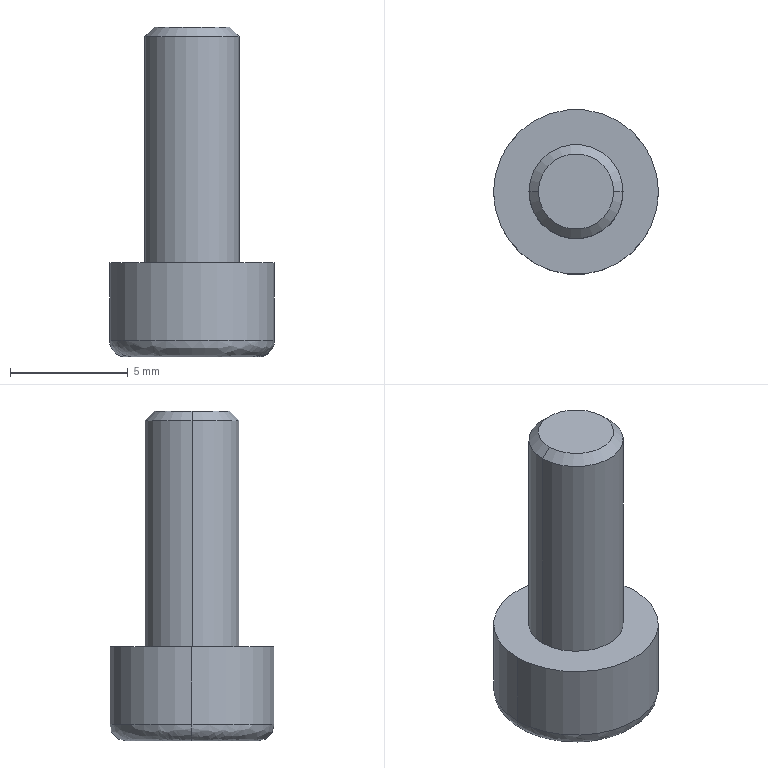Part | STEP file | LE-YZS-M4X10_PN_0007 | 1 solid | 25 faces | box 7 x 7 x 14 mm | volume 258.83 mm3 | plane 15 | cylinder 4 | cone 4 | spline 2 | commonest cylinder face diameters 4 x2 7 x2
STEP:
#1=CARTESIAN_POINT('',(-3.5,0.,-3.3));
#2=VERTEX_POINT('',#1);
#3=CARTESIAN_POINT('',(3.5,0.,-3.3));
#4=VERTEX_POINT('',#3);
#5=CARTESIAN_POINT('',(0.,0.,-3.3));
#6=DIRECTION('',(0.,0.,1.));
#7=DIRECTION('',(1.,0.,0.));
#8=AXIS2_PLACEMENT_3D('',#5,#6,#7);
#9=CIRCLE('',#8,3.5);
#10=EDGE_CURVE('',#2,#4,#9,.T.);
#11=ORIENTED_EDGE('',*,*,#10,.F.);
#12=CARTESIAN_POINT('',(-2.8,0.,-4.));
#13=VERTEX_POINT('',#12);
#14=CARTESIAN_POINT('',(-2.8,0.,-3.3));
#15=DIRECTION('',(0.,-1.,0.));
#16=DIRECTION('',(-1.,0.,0.));
#17=AXIS2_PLACEMENT_3D('',#14,#15,#16);
#18=CIRCLE('',#17,0.7);
#19=EDGE_CURVE('',#2,#13,#18,.T.);
#20=ORIENTED_EDGE('',*,*,#19,.T.);
#21=CARTESIAN_POINT('',(2.8,0.,-4.));
#22=VERTEX_POINT('',#21);
#23=CARTESIAN_POINT('',(-2.8,0.,-4.));
#24=CARTESIAN_POINT('',(-2.8,-5.6,-4.));
#25=CARTESIAN_POINT('',(2.8,-5.6,-4.));
#26=CARTESIAN_POINT('',(2.8,0.,-4.));
#27=(BOUNDED_CURVE()B_SPLINE_CURVE(3,(#23,#24,#25,#26),.UNSPECIFIED.,.F.,.F.)B_SPLINE_CURVE_WITH_KNOTS((4,4),(0.,1.),.UNSPECIFIED.)CURVE()GEOMETRIC_REPRESENTATION_ITEM()RATIONAL_B_SPLINE_CURVE((1.,0.3333,0.3333,1.))REPRESENTATION_ITEM(''));
#28=EDGE_CURVE('',#13,#22,#27,.T.);
#29=ORIENTED_EDGE('',*,*,#28,.T.);
#30=CARTESIAN_POINT('',(2.8,0.,-3.3));
#31=DIRECTION('',(0.,1.,0.));
#32=DIRECTION('',(1.,0.,0.));
#33=AXIS2_PLACEMENT_3D('',#30,#31,#32);
#34=CIRCLE('',#33,0.7);
#35=EDGE_CURVE('',#4,#22,#34,.T.);
#36=ORIENTED_EDGE('',*,*,#35,.F.);
#37=EDGE_LOOP('',(#11,#20,#29,#36));
#38=FACE_OUTER_BOUND('',#37,.T.);
#39=CARTESIAN_POINT('',(-3.5,0.,-3.3));
#40=CARTESIAN_POINT('',(-3.5,-7.,-3.3));
#41=CARTESIAN_POINT('',(3.5,-7.,-3.3));
#42=CARTESIAN_POINT('',(3.5,0.,-3.3));
#43=CARTESIAN_POINT('',(-3.5,0.,-3.71));
#44=CARTESIAN_POINT('',(-3.5,-7.,-3.71));
#45=CARTESIAN_POINT('',(3.5,-7.,-3.71));
#46=CARTESIAN_POINT('',(3.5,0.,-3.71));
#47=CARTESIAN_POINT('',(-3.21,0.,-4.));
#48=CARTESIAN_POINT('',(-3.21,-6.42,-4.));
#49=CARTESIAN_POINT('',(3.21,-6.42,-4.));
#50=CARTESIAN_POINT('',(3.21,0.,-4.));
#51=CARTESIAN_POINT('',(-2.8,0.,-4.));
#52=CARTESIAN_POINT('',(-2.8,-5.6,-4.));
#53=CARTESIAN_POINT('',(2.8,-5.6,-4.));
#54=CARTESIAN_POINT('',(2.8,0.,-4.));
#55=(BOUNDED_SURFACE()B_SPLINE_SURFACE(3,3,((#39,#40,#41,#42),(#43,#44,#45,#46),(#47,#48,#49,#50),(#51,#52,#53,#54)),.UNSPECIFIED.,.F.,.F.,.T.)B_SPLINE_SURFACE_WITH_KNOTS((4,4),(4,4),(0.,1.),(0.,1.),.UNSPECIFIED.)GEOMETRIC_REPRESENTATION_ITEM()RATIONAL_B_SPLINE_SURFACE(((1.,0.3333,0.3333,1.),(0.8047,0.2682,0.2682,0.8047),(0.8047,0.2682,0.2682,0.8047),(1.,0.3333,0.3333,1.)))REPRESENTATION_ITEM('')SURFACE());
#56=ADVANCED_FACE('',(#38),#55,.T.);
#57=CARTESIAN_POINT('',(-2.,0.,9.6));
#58=VERTEX_POINT('',#57);
#59=CARTESIAN_POINT('',(2.,0.,9.6));
#60=VERTEX_POINT('',#59);
#61=CARTESIAN_POINT('',(0.,0.,9.6));
#62=DIRECTION('',(0.,0.,-1.));
#63=DIRECTION('',(-1.,0.,0.));
#64=AXIS2_PLACEMENT_3D('',#61,#62,#63);
#65=CIRCLE('',#64,2.);
#66=EDGE_CURVE('',#58,#60,#65,.T.);
#67=ORIENTED_EDGE('',*,*,#66,.T.);
#68=CARTESIAN_POINT('',(2.,0.,0.));
#69=VERTEX_POINT('',#68);
#70=CARTESIAN_POINT('',(2.,0.,10.));
#71=DIRECTION('',(0.,0.,-1.));
#72=VECTOR('',#71,1000.);
#73=LINE('',#70,#72);
#74=EDGE_CURVE('',#60,#69,#73,.T.);
#75=ORIENTED_EDGE('',*,*,#74,.T.);
#76=CARTESIAN_POINT('',(-2.,0.,0.));
#77=VERTEX_POINT('',#76);
#78=CARTESIAN_POINT('',(0.,0.,0.));
#79=DIRECTION('',(0.,0.,1.));
#80=DIRECTION('',(-1.,0.,0.));
#81=AXIS2_PLACEMENT_3D('',#78,#79,#80);
#82=CIRCLE('',#81,2.);
#83=EDGE_CURVE('',#69,#77,#82,.T.);
#84=ORIENTED_EDGE('',*,*,#83,.T.);
#85=CARTESIAN_POINT('',(-2.,0.,10.));
#86=DIRECTION('',(0.,0.,-1.));
#87=VECTOR('',#86,1000.);
#88=LINE('',#85,#87);
#89=EDGE_CURVE('',#58,#77,#88,.T.);
#90=ORIENTED_EDGE('',*,*,#89,.F.);
#91=EDGE_LOOP('',(#67,#75,#84,#90));
#92=FACE_OUTER_BOUND('',#91,.T.);
#93=CARTESIAN_POINT('',(0.,0.,10.));
#94=DIRECTION('',(0.,0.,-1.));
#95=DIRECTION('',(-1.,0.,0.));
#96=AXIS2_PLACEMENT_3D('',#93,#94,#95);
#97=CYLINDRICAL_SURFACE('',#96,2.);
#98=ADVANCED_FACE('',(#92),#97,.T.);
#99=CARTESIAN_POINT('',(-1.6,0.,10.));
#100=VERTEX_POINT('',#99);
#101=CARTESIAN_POINT('',(1.6,0.,10.));
#102=VERTEX_POINT('',#101);
#103=CARTESIAN_POINT('',(0.,0.,10.));
#104=DIRECTION('',(0.,0.,-1.));
#105=DIRECTION('',(-1.,0.,0.));
#106=AXIS2_PLACEMENT_3D('',#103,#104,#105);
#107=CIRCLE('',#106,1.6);
#108=EDGE_CURVE('',#100,#102,#107,.T.);
#109=ORIENTED_EDGE('',*,*,#108,.T.);
#110=CARTESIAN_POINT('',(2.,0.,9.6));
#111=DIRECTION('',(0.7071,0.,-0.7071));
#112=VECTOR('',#111,1000.);
#113=LINE('',#110,#112);
#114=EDGE_CURVE('',#102,#60,#113,.T.);
#115=ORIENTED_EDGE('',*,*,#114,.T.);
#116=ORIENTED_EDGE('',*,*,#66,.F.);
#117=CARTESIAN_POINT('',(-2.,0.,9.6));
#118=DIRECTION('',(-0.7071,0.,-0.7071));
#119=VECTOR('',#118,1000.);
#120=LINE('',#117,#119);
#121=EDGE_CURVE('',#100,#58,#120,.T.);
#122=ORIENTED_EDGE('',*,*,#121,.F.);
#123=EDGE_LOOP('',(#109,#115,#116,#122));
#124=FACE_OUTER_BOUND('',#123,.T.);
#125=CARTESIAN_POINT('',(0.,0.,9.6));
#126=DIRECTION('',(0.,0.,-1.));
#127=DIRECTION('',(-1.,0.,0.));
#128=AXIS2_PLACEMENT_3D('',#125,#126,#127);
#129=CONICAL_SURFACE('',#128,2.,0.7854);
#130=ADVANCED_FACE('',(#124),#129,.T.);
#131=CARTESIAN_POINT('',(0.,0.,-3.3));
#132=DIRECTION('',(0.,0.,1.));
#133=DIRECTION('',(1.,0.,0.));
#134=AXIS2_PLACEMENT_3D('',#131,#132,#133);
#135=CIRCLE('',#134,3.5);
#136=EDGE_CURVE('',#4,#2,#135,.T.);
#137=ORIENTED_EDGE('',*,*,#136,.T.);
#138=CARTESIAN_POINT('',(-3.5,0.,0.));
#139=VERTEX_POINT('',#138);
#140=CARTESIAN_POINT('',(-3.5,0.,-4.));
#141=DIRECTION('',(0.,0.,1.));
#142=VECTOR('',#141,1000.);
#143=LINE('',#140,#142);
#144=EDGE_CURVE('',#2,#139,#143,.T.);
#145=ORIENTED_EDGE('',*,*,#144,.T.);
#146=CARTESIAN_POINT('',(3.5,0.,0.));
#147=VERTEX_POINT('',#146);
#148=CARTESIAN_POINT('',(0.,0.,0.));
#149=DIRECTION('',(0.,0.,1.));
#150=DIRECTION('',(1.,0.,0.));
#151=AXIS2_PLACEMENT_3D('',#148,#149,#150);
#152=CIRCLE('',#151,3.5);
#153=EDGE_CURVE('',#147,#139,#152,.T.);
#154=ORIENTED_EDGE('',*,*,#153,.F.);
#155=CARTESIAN_POINT('',(3.5,0.,-4.));
#156=DIRECTION('',(0.,0.,1.));
#157=VECTOR('',#156,1000.);
#158=LINE('',#155,#157);
#159=EDGE_CURVE('',#4,#147,#158,.T.);
#160=ORIENTED_EDGE('',*,*,#159,.F.);
#161=EDGE_LOOP('',(#137,#145,#154,#160));
#162=FACE_OUTER_BOUND('',#161,.T.);
#163=CARTESIAN_POINT('',(0.,0.,-4.));
#164=DIRECTION('',(0.,0.,1.));
#165=DIRECTION('',(1.,0.,0.));
#166=AXIS2_PLACEMENT_3D('',#163,#164,#165);
#167=CYLINDRICAL_SURFACE('',#166,3.5);
#168=ADVANCED_FACE('',(#162),#167,.T.);
#169=CARTESIAN_POINT('',(0.,0.,-1.134));
#170=VERTEX_POINT('',#169);
#171=CARTESIAN_POINT('',(-1.5,0.,-2.));
#172=VERTEX_POINT('',#171);
#173=CARTESIAN_POINT('',(-1.5,0.,-2.));
#174=DIRECTION('',(-0.866,0.,-0.5));
#175=VECTOR('',#174,1000.);
#176=LINE('',#173,#175);
#177=EDGE_CURVE('',#170,#172,#176,.T.);
#178=ORIENTED_EDGE('',*,*,#177,.F.);
#179=CARTESIAN_POINT('',(1.5,0.,-2.));
#180=VERTEX_POINT('',#179);
#181=CARTESIAN_POINT('',(1.5,0.,-2.));
#182=DIRECTION('',(0.866,0.,-0.5));
#183=VECTOR('',#182,1000.);
#184=LINE('',#181,#183);
#185=EDGE_CURVE('',#170,#180,#184,.T.);
#186=ORIENTED_EDGE('',*,*,#185,.T.);
#187=CARTESIAN_POINT('',(1.299,-0.75,-2.));
#188=VERTEX_POINT('',#187);
#189=CARTESIAN_POINT('',(0.,0.,-2.));
#190=DIRECTION('',(0.,0.,-1.));
#191=DIRECTION('',(-1.,0.,0.));
#192=AXIS2_PLACEMENT_3D('',#189,#190,#191);
#193=CIRCLE('',#192,1.5);
#194=EDGE_CURVE('',#180,#188,#193,.T.);
#195=ORIENTED_EDGE('',*,*,#194,.T.);
#196=CARTESIAN_POINT('',(0.,-1.5,-2.));
#197=VERTEX_POINT('',#196);
#198=CARTESIAN_POINT('',(0.,0.,-2.));
#199=DIRECTION('',(0.,0.,-1.));
#200=DIRECTION('',(-1.,0.,0.));
#201=AXIS2_PLACEMENT_3D('',#198,#199,#200);
#202=CIRCLE('',#201,1.5);
#203=EDGE_CURVE('',#188,#197,#202,.T.);
#204=ORIENTED_EDGE('',*,*,#203,.T.);
#205=CARTESIAN_POINT('',(-1.299,-0.75,-2.));
#206=VERTEX_POINT('',#205);
#207=CARTESIAN_POINT('',(0.,0.,-2.));
#208=DIRECTION('',(0.,0.,1.));
#209=DIRECTION('',(-1.,0.,0.));
#210=AXIS2_PLACEMENT_3D('',#207,#208,#209);
#211=CIRCLE('',#210,1.5);
#212=EDGE_CURVE('',#206,#197,#211,.T.);
#213=ORIENTED_EDGE('',*,*,#212,.F.);
#214=CARTESIAN_POINT('',(0.,0.,-2.));
#215=DIRECTION('',(0.,0.,1.));
#216=DIRECTION('',(-1.,0.,0.));
#217=AXIS2_PLACEMENT_3D('',#214,#215,#216);
#218=CIRCLE('',#217,1.5);
#219=EDGE_CURVE('',#172,#206,#218,.T.);
#220=ORIENTED_EDGE('',*,*,#219,.F.);
#221=EDGE_LOOP('',(#178,#186,#195,#204,#213,#220));
#222=FACE_OUTER_BOUND('',#221,.T.);
#223=CARTESIAN_POINT('',(0.,0.,-2.));
#224=DIRECTION('',(0.,0.,-1.));
#225=DIRECTION('',(-1.,0.,0.));
#226=AXIS2_PLACEMENT_3D('',#223,#224,#225);
#227=CONICAL_SURFACE('',#226,1.5,1.047);
#228=ADVANCED_FACE('',(#222),#227,.F.);
#229=ORIENTED_EDGE('',*,*,#74,.F.);
#230=CARTESIAN_POINT('',(0.,0.,9.6));
#231=DIRECTION('',(0.,0.,-1.));
#232=DIRECTION('',(-1.,0.,0.));
#233=AXIS2_PLACEMENT_3D('',#230,#231,#232);
#234=CIRCLE('',#233,2.);
#235=EDGE_CURVE('',#60,#58,#234,.T.);
#236=ORIENTED_EDGE('',*,*,#235,.T.);
#237=ORIENTED_EDGE('',*,*,#89,.T.);
#238=CARTESIAN_POINT('',(0.,0.,0.));
#239=DIRECTION('',(0.,0.,1.));
#240=DIRECTION('',(-1.,0.,0.));
#241=AXIS2_PLACEMENT_3D('',#238,#239,#240);
#242=CIRCLE('',#241,2.);
#243=EDGE_CURVE('',#77,#69,#242,.T.);
#244=ORIENTED_EDGE('',*,*,#243,.T.);
#245=EDGE_LOOP('',(#229,#236,#237,#244));
#246=FACE_OUTER_BOUND('',#245,.T.);
#247=CARTESIAN_POINT('',(0.,0.,10.));
#248=DIRECTION('',(0.,0.,-1.));
#249=DIRECTION('',(-1.,0.,0.));
#250=AXIS2_PLACEMENT_3D('',#247,#248,#249);
#251=CYLINDRICAL_SURFACE('',#250,2.);
#252=ADVANCED_FACE('',(#246),#251,.T.);
#253=ORIENTED_EDGE('',*,*,#153,.T.);
#254=CARTESIAN_POINT('',(0.,0.,0.));
#255=DIRECTION('',(0.,0.,1.));
#256=DIRECTION('',(1.,0.,0.));
#257=AXIS2_PLACEMENT_3D('',#254,#255,#256);
#258=CIRCLE('',#257,3.5);
#259=EDGE_CURVE('',#139,#147,#258,.T.);
#260=ORIENTED_EDGE('',*,*,#259,.T.);
#261=EDGE_LOOP('',(#253,#260));
#262=FACE_OUTER_BOUND('',#261,.T.);
#263=ORIENTED_EDGE('',*,*,#243,.F.);
#264=ORIENTED_EDGE('',*,*,#83,.F.);
#265=EDGE_LOOP('',(#263,#264));
#266=FACE_BOUND('',#265,.T.);
#267=CARTESIAN_POINT('',(0.,0.,0.));
#268=DIRECTION('',(0.,0.,1.));
#269=DIRECTION('',(1.,0.,0.));
#270=AXIS2_PLACEMENT_3D('',#267,#268,#269);
#271=PLANE('',#270);
#272=ADVANCED_FACE('',(#262,#266),#271,.T.);
#273=ORIENTED_EDGE('',*,*,#114,.F.);
#274=CARTESIAN_POINT('',(0.,0.,10.));
#275=DIRECTION('',(0.,0.,-1.));
#276=DIRECTION('',(-1.,0.,0.));
#277=AXIS2_PLACEMENT_3D('',#274,#275,#276);
#278=CIRCLE('',#277,1.6);
#279=EDGE_CURVE('',#102,#100,#278,.T.);
#280=ORIENTED_EDGE('',*,*,#279,.T.);
#281=ORIENTED_EDGE('',*,*,#121,.T.);
#282=ORIENTED_EDGE('',*,*,#235,.F.);
#283=EDGE_LOOP('',(#273,#280,#281,#282));
#284=FACE_OUTER_BOUND('',#283,.T.);
#285=CARTESIAN_POINT('',(0.,0.,9.6));
#286=DIRECTION('',(0.,0.,-1.));
#287=DIRECTION('',(-1.,0.,0.));
#288=AXIS2_PLACEMENT_3D('',#285,#286,#287);
#289=CONICAL_SURFACE('',#288,2.,0.7854);
#290=ADVANCED_FACE('',(#284),#289,.T.);
#291=ORIENTED_EDGE('',*,*,#144,.F.);
#292=ORIENTED_EDGE('',*,*,#10,.T.);
#293=ORIENTED_EDGE('',*,*,#159,.T.);
#294=ORIENTED_EDGE('',*,*,#259,.F.);
#295=EDGE_LOOP('',(#291,#292,#293,#294));
#296=FACE_OUTER_BOUND('',#295,.T.);
#297=CARTESIAN_POINT('',(0.,0.,-4.));
#298=DIRECTION('',(0.,0.,1.));
#299=DIRECTION('',(1.,0.,0.));
#300=AXIS2_PLACEMENT_3D('',#297,#298,#299);
#301=CYLINDRICAL_SURFACE('',#300,3.5);
#302=ADVANCED_FACE('',(#296),#301,.T.);
#303=ORIENTED_EDGE('',*,*,#108,.F.);
#304=ORIENTED_EDGE('',*,*,#279,.F.);
#305=EDGE_LOOP('',(#303,#304));
#306=FACE_OUTER_BOUND('',#305,.T.);
#307=CARTESIAN_POINT('',(0.,0.,10.));
#308=DIRECTION('',(0.,0.,-1.));
#309=DIRECTION('',(-1.,0.,0.));
#310=AXIS2_PLACEMENT_3D('',#307,#308,#309);
#311=PLANE('',#310);
#312=ADVANCED_FACE('',(#306),#311,.F.);
#313=ORIENTED_EDGE('',*,*,#19,.F.);
#314=ORIENTED_EDGE('',*,*,#136,.F.);
#315=ORIENTED_EDGE('',*,*,#35,.T.);
#316=CARTESIAN_POINT('',(2.8,0.,-4.));
#317=CARTESIAN_POINT('',(2.8,5.6,-4.));
#318=CARTESIAN_POINT('',(-2.8,5.6,-4.));
#319=CARTESIAN_POINT('',(-2.8,0.,-4.));
#320=(BOUNDED_CURVE()B_SPLINE_CURVE(3,(#316,#317,#318,#319),.UNSPECIFIED.,.F.,.T.)B_SPLINE_CURVE_WITH_KNOTS((4,4),(0.,1.),.UNSPECIFIED.)CURVE()GEOMETRIC_REPRESENTATION_ITEM()RATIONAL_B_SPLINE_CURVE((1.,0.3333,0.3333,1.))REPRESENTATION_ITEM(''));
#321=EDGE_CURVE('',#22,#13,#320,.T.);
#322=ORIENTED_EDGE('',*,*,#321,.T.);
#323=EDGE_LOOP('',(#313,#314,#315,#322));
#324=FACE_OUTER_BOUND('',#323,.T.);
#325=CARTESIAN_POINT('',(3.5,0.,-3.3));
#326=CARTESIAN_POINT('',(3.5,7.,-3.3));
#327=CARTESIAN_POINT('',(-3.5,7.,-3.3));
#328=CARTESIAN_POINT('',(-3.5,0.,-3.3));
#329=CARTESIAN_POINT('',(3.5,0.,-3.71));
#330=CARTESIAN_POINT('',(3.5,7.,-3.71));
#331=CARTESIAN_POINT('',(-3.5,7.,-3.71));
#332=CARTESIAN_POINT('',(-3.5,0.,-3.71));
#333=CARTESIAN_POINT('',(3.21,0.,-4.));
#334=CARTESIAN_POINT('',(3.21,6.42,-4.));
#335=CARTESIAN_POINT('',(-3.21,6.42,-4.));
#336=CARTESIAN_POINT('',(-3.21,0.,-4.));
#337=CARTESIAN_POINT('',(2.8,0.,-4.));
#338=CARTESIAN_POINT('',(2.8,5.6,-4.));
#339=CARTESIAN_POINT('',(-2.8,5.6,-4.));
#340=CARTESIAN_POINT('',(-2.8,0.,-4.));
#341=(BOUNDED_SURFACE()B_SPLINE_SURFACE(3,3,((#325,#326,#327,#328),(#329,#330,#331,#332),(#333,#334,#335,#336),(#337,#338,#339,#340)),.UNSPECIFIED.,.F.,.F.,.F.)B_SPLINE_SURFACE_WITH_KNOTS((4,4),(4,4),(0.,1.),(0.,1.),.UNSPECIFIED.)GEOMETRIC_REPRESENTATION_ITEM()RATIONAL_B_SPLINE_SURFACE(((1.,0.3333,0.3333,1.),(0.8047,0.2682,0.2682,0.8047),(0.8047,0.2682,0.2682,0.8047),(1.,0.3333,0.3333,1.)))REPRESENTATION_ITEM('')SURFACE());
#342=ADVANCED_FACE('',(#324),#341,.T.);
#343=CARTESIAN_POINT('',(-0.866,1.5,-4.));
#344=VERTEX_POINT('',#343);
#345=CARTESIAN_POINT('',(0.866,1.5,-4.));
#346=VERTEX_POINT('',#345);
#347=CARTESIAN_POINT('',(0.866,1.5,-4.));
#348=DIRECTION('',(1.,0.,0.));
#349=VECTOR('',#348,1000.);
#350=LINE('',#347,#349);
#351=EDGE_CURVE('',#344,#346,#350,.T.);
#352=ORIENTED_EDGE('',*,*,#351,.F.);
#353=CARTESIAN_POINT('',(-1.732,0.,-4.));
#354=VERTEX_POINT('',#353);
#355=CARTESIAN_POINT('',(-0.866,1.5,-4.));
#356=DIRECTION('',(0.5,0.866,0.));
#357=VECTOR('',#356,1000.);
#358=LINE('',#355,#357);
#359=EDGE_CURVE('',#354,#344,#358,.T.);
#360=ORIENTED_EDGE('',*,*,#359,.F.);
#361=CARTESIAN_POINT('',(-0.866,-1.5,-4.));
#362=VERTEX_POINT('',#361);
#363=CARTESIAN_POINT('',(-1.732,0.,-4.));
#364=DIRECTION('',(-0.5,0.866,0.));
#365=VECTOR('',#364,1000.);
#366=LINE('',#363,#365);
#367=EDGE_CURVE('',#362,#354,#366,.T.);
#368=ORIENTED_EDGE('',*,*,#367,.F.);
#369=CARTESIAN_POINT('',(0.866,-1.5,-4.));
#370=VERTEX_POINT('',#369);
#371=CARTESIAN_POINT('',(-0.866,-1.5,-4.));
#372=DIRECTION('',(-1.,0.,0.));
#373=VECTOR('',#372,1000.);
#374=LINE('',#371,#373);
#375=EDGE_CURVE('',#370,#362,#374,.T.);
#376=ORIENTED_EDGE('',*,*,#375,.F.);
#377=CARTESIAN_POINT('',(1.732,0.,-4.));
#378=VERTEX_POINT('',#377);
#379=CARTESIAN_POINT('',(0.866,-1.5,-4.));
#380=DIRECTION('',(-0.5,-0.866,0.));
#381=VECTOR('',#380,1000.);
#382=LINE('',#379,#381);
#383=EDGE_CURVE('',#378,#370,#382,.T.);
#384=ORIENTED_EDGE('',*,*,#383,.F.);
#385=CARTESIAN_POINT('',(0.866,1.5,-4.));
#386=DIRECTION('',(0.5,-0.866,0.));
#387=VECTOR('',#386,1000.);
#388=LINE('',#385,#387);
#389=EDGE_CURVE('',#346,#378,#388,.T.);
#390=ORIENTED_EDGE('',*,*,#389,.F.);
#391=EDGE_LOOP('',(#352,#360,#368,#376,#384,#390));
#392=FACE_BOUND('',#391,.T.);
#393=ORIENTED_EDGE('',*,*,#321,.F.);
#394=ORIENTED_EDGE('',*,*,#28,.F.);
#395=EDGE_LOOP('',(#393,#394));
#396=FACE_OUTER_BOUND('',#395,.T.);
#397=CARTESIAN_POINT('',(0.,0.,-4.));
#398=DIRECTION('',(0.,0.,1.));
#399=DIRECTION('',(1.,0.,0.));
#400=AXIS2_PLACEMENT_3D('',#397,#398,#399);
#401=PLANE('',#400);
#402=ADVANCED_FACE('',(#392,#396),#401,.F.);
#403=CARTESIAN_POINT('',(1.299,0.75,-2.));
#404=VERTEX_POINT('',#403);
#405=CARTESIAN_POINT('',(0.866,1.5,-2.));
#406=VERTEX_POINT('',#405);
#407=CARTESIAN_POINT('',(1.732,0.,-2.));
#408=DIRECTION('',(-0.5,0.866,0.));
#409=VECTOR('',#408,1000.);
#410=LINE('',#407,#409);
#411=EDGE_CURVE('',#404,#406,#410,.T.);
#412=ORIENTED_EDGE('',*,*,#411,.T.);
#413=CARTESIAN_POINT('',(0.866,1.5,-2.));
#414=DIRECTION('',(0.,0.,-1.));
#415=VECTOR('',#414,1000.);
#416=LINE('',#413,#415);
#417=EDGE_CURVE('',#406,#346,#416,.T.);
#418=ORIENTED_EDGE('',*,*,#417,.T.);
#419=ORIENTED_EDGE('',*,*,#389,.T.);
#420=CARTESIAN_POINT('',(1.732,0.,-2.));
#421=VERTEX_POINT('',#420);
#422=CARTESIAN_POINT('',(1.732,0.,-2.));
#423=DIRECTION('',(0.,0.,1.));
#424=VECTOR('',#423,1000.);
#425=LINE('',#422,#424);
#426=EDGE_CURVE('',#378,#421,#425,.T.);
#427=ORIENTED_EDGE('',*,*,#426,.T.);
#428=CARTESIAN_POINT('',(1.732,0.,-2.));
#429=DIRECTION('',(-0.5,0.866,0.));
#430=VECTOR('',#429,1000.);
#431=LINE('',#428,#430);
#432=EDGE_CURVE('',#421,#404,#431,.T.);
#433=ORIENTED_EDGE('',*,*,#432,.T.);
#434=EDGE_LOOP('',(#412,#418,#419,#427,#433));
#435=FACE_OUTER_BOUND('',#434,.T.);
#436=CARTESIAN_POINT('',(1.732,0.,-2.));
#437=DIRECTION('',(-0.866,-0.5,0.));
#438=DIRECTION('',(0.5,-0.866,0.));
#439=AXIS2_PLACEMENT_3D('',#436,#437,#438);
#440=PLANE('',#439);
#441=ADVANCED_FACE('',(#435),#440,.T.);
#442=CARTESIAN_POINT('',(0.,1.5,-2.));
#443=VERTEX_POINT('',#442);
#444=CARTESIAN_POINT('',(-0.866,1.5,-2.));
#445=VERTEX_POINT('',#444);
#446=CARTESIAN_POINT('',(0.866,1.5,-2.));
#447=DIRECTION('',(-1.,0.,0.));
#448=VECTOR('',#447,1000.);
#449=LINE('',#446,#448);
#450=EDGE_CURVE('',#443,#445,#449,.T.);
#451=ORIENTED_EDGE('',*,*,#450,.T.);
#452=CARTESIAN_POINT('',(-0.866,1.5,-2.));
#453=DIRECTION('',(0.,0.,-1.));
#454=VECTOR('',#453,1000.);
#455=LINE('',#452,#454);
#456=EDGE_CURVE('',#445,#344,#455,.T.);
#457=ORIENTED_EDGE('',*,*,#456,.T.);
#458=ORIENTED_EDGE('',*,*,#351,.T.);
#459=ORIENTED_EDGE('',*,*,#417,.F.);
#460=CARTESIAN_POINT('',(0.866,1.5,-2.));
#461=DIRECTION('',(-1.,0.,0.));
#462=VECTOR('',#461,1000.);
#463=LINE('',#460,#462);
#464=EDGE_CURVE('',#406,#443,#463,.T.);
#465=ORIENTED_EDGE('',*,*,#464,.T.);
#466=EDGE_LOOP('',(#451,#457,#458,#459,#465));
#467=FACE_OUTER_BOUND('',#466,.T.);
#468=CARTESIAN_POINT('',(0.866,1.5,-2.));
#469=DIRECTION('',(0.,-1.,0.));
#470=DIRECTION('',(1.,0.,0.));
#471=AXIS2_PLACEMENT_3D('',#468,#469,#470);
#472=PLANE('',#471);
#473=ADVANCED_FACE('',(#467),#472,.T.);
#474=CARTESIAN_POINT('',(0.,0.,-2.));
#475=DIRECTION('',(0.,0.,-1.));
#476=DIRECTION('',(-1.,0.,0.));
#477=AXIS2_PLACEMENT_3D('',#474,#475,#476);
#478=CIRCLE('',#477,1.5);
#479=EDGE_CURVE('',#443,#404,#478,.T.);
#480=ORIENTED_EDGE('',*,*,#479,.F.);
#481=ORIENTED_EDGE('',*,*,#464,.F.);
#482=ORIENTED_EDGE('',*,*,#411,.F.);
#483=EDGE_LOOP('',(#480,#481,#482));
#484=FACE_OUTER_BOUND('',#483,.T.);
#485=CARTESIAN_POINT('',(0.,0.,-2.));
#486=DIRECTION('',(0.,0.,1.));
#487=DIRECTION('',(1.,0.,0.));
#488=AXIS2_PLACEMENT_3D('',#485,#486,#487);
#489=PLANE('',#488);
#490=ADVANCED_FACE('',(#484),#489,.F.);
#491=CARTESIAN_POINT('',(1.299,-0.75,-2.));
#492=DIRECTION('',(0.5,0.866,0.));
#493=VECTOR('',#492,1000.);
#494=LINE('',#491,#493);
#495=EDGE_CURVE('',#188,#421,#494,.T.);
#496=ORIENTED_EDGE('',*,*,#495,.F.);
#497=ORIENTED_EDGE('',*,*,#194,.F.);
#498=CARTESIAN_POINT('',(0.,0.,-2.));
#499=DIRECTION('',(0.,0.,-1.));
#500=DIRECTION('',(-1.,0.,0.));
#501=AXIS2_PLACEMENT_3D('',#498,#499,#500);
#502=CIRCLE('',#501,1.5);
#503=EDGE_CURVE('',#404,#180,#502,.T.);
#504=ORIENTED_EDGE('',*,*,#503,.F.);
#505=ORIENTED_EDGE('',*,*,#432,.F.);
#506=EDGE_LOOP('',(#496,#497,#504,#505));
#507=FACE_OUTER_BOUND('',#506,.T.);
#508=CARTESIAN_POINT('',(0.,0.,-2.));
#509=DIRECTION('',(0.,0.,1.));
#510=DIRECTION('',(1.,0.,0.));
#511=AXIS2_PLACEMENT_3D('',#508,#509,#510);
#512=PLANE('',#511);
#513=ADVANCED_FACE('',(#507),#512,.F.);
#514=ORIENTED_EDGE('',*,*,#495,.T.);
#515=ORIENTED_EDGE('',*,*,#426,.F.);
#516=ORIENTED_EDGE('',*,*,#383,.T.);
#517=CARTESIAN_POINT('',(0.866,-1.5,-2.));
#518=VERTEX_POINT('',#517);
#519=CARTESIAN_POINT('',(0.866,-1.5,-2.));
#520=DIRECTION('',(0.,0.,1.));
#521=VECTOR('',#520,1000.);
#522=LINE('',#519,#521);
#523=EDGE_CURVE('',#370,#518,#522,.T.);
#524=ORIENTED_EDGE('',*,*,#523,.T.);
#525=CARTESIAN_POINT('',(0.866,-1.5,-2.));
#526=DIRECTION('',(0.5,0.866,0.));
#527=VECTOR('',#526,1000.);
#528=LINE('',#525,#527);
#529=EDGE_CURVE('',#518,#188,#528,.T.);
#530=ORIENTED_EDGE('',*,*,#529,.T.);
#531=EDGE_LOOP('',(#514,#515,#516,#524,#530));
#532=FACE_OUTER_BOUND('',#531,.T.);
#533=CARTESIAN_POINT('',(0.866,-1.5,-2.));
#534=DIRECTION('',(-0.866,0.5,0.));
#535=DIRECTION('',(-0.5,-0.866,0.));
#536=AXIS2_PLACEMENT_3D('',#533,#534,#535);
#537=PLANE('',#536);
#538=ADVANCED_FACE('',(#532),#537,.T.);
#539=CARTESIAN_POINT('',(-1.299,0.75,-2.));
#540=VERTEX_POINT('',#539);
#541=CARTESIAN_POINT('',(-1.732,0.,-2.));
#542=VERTEX_POINT('',#541);
#543=CARTESIAN_POINT('',(-0.866,1.5,-2.));
#544=DIRECTION('',(-0.5,-0.866,0.));
#545=VECTOR('',#544,1000.);
#546=LINE('',#543,#545);
#547=EDGE_CURVE('',#540,#542,#546,.T.);
#548=ORIENTED_EDGE('',*,*,#547,.T.);
#549=CARTESIAN_POINT('',(-1.732,0.,-2.));
#550=DIRECTION('',(0.,0.,-1.));
#551=VECTOR('',#550,1000.);
#552=LINE('',#549,#551);
#553=EDGE_CURVE('',#542,#354,#552,.T.);
#554=ORIENTED_EDGE('',*,*,#553,.T.);
#555=ORIENTED_EDGE('',*,*,#359,.T.);
#556=ORIENTED_EDGE('',*,*,#456,.F.);
#557=CARTESIAN_POINT('',(-0.866,1.5,-2.));
#558=DIRECTION('',(-0.5,-0.866,0.));
#559=VECTOR('',#558,1000.);
#560=LINE('',#557,#559);
#561=EDGE_CURVE('',#445,#540,#560,.T.);
#562=ORIENTED_EDGE('',*,*,#561,.T.);
#563=EDGE_LOOP('',(#548,#554,#555,#556,#562));
#564=FACE_OUTER_BOUND('',#563,.T.);
#565=CARTESIAN_POINT('',(-0.866,1.5,-2.));
#566=DIRECTION('',(0.866,-0.5,0.));
#567=DIRECTION('',(0.5,0.866,0.));
#568=AXIS2_PLACEMENT_3D('',#565,#566,#567);
#569=PLANE('',#568);
#570=ADVANCED_FACE('',(#564),#569,.T.);
#571=CARTESIAN_POINT('',(0.,0.,-2.));
#572=DIRECTION('',(0.,0.,-1.));
#573=DIRECTION('',(-1.,0.,0.));
#574=AXIS2_PLACEMENT_3D('',#571,#572,#573);
#575=CIRCLE('',#574,1.5);
#576=EDGE_CURVE('',#540,#443,#575,.T.);
#577=ORIENTED_EDGE('',*,*,#576,.F.);
#578=ORIENTED_EDGE('',*,*,#561,.F.);
#579=ORIENTED_EDGE('',*,*,#450,.F.);
#580=EDGE_LOOP('',(#577,#578,#579));
#581=FACE_OUTER_BOUND('',#580,.T.);
#582=CARTESIAN_POINT('',(0.,0.,-2.));
#583=DIRECTION('',(0.,0.,1.));
#584=DIRECTION('',(1.,0.,0.));
#585=AXIS2_PLACEMENT_3D('',#582,#583,#584);
#586=PLANE('',#585);
#587=ADVANCED_FACE('',(#581),#586,.F.);
#588=ORIENTED_EDGE('',*,*,#185,.F.);
#589=ORIENTED_EDGE('',*,*,#177,.T.);
#590=CARTESIAN_POINT('',(0.,0.,-2.));
#591=DIRECTION('',(0.,0.,1.));
#592=DIRECTION('',(-1.,0.,0.));
#593=AXIS2_PLACEMENT_3D('',#590,#591,#592);
#594=CIRCLE('',#593,1.5);
#595=EDGE_CURVE('',#540,#172,#594,.T.);
#596=ORIENTED_EDGE('',*,*,#595,.F.);
#597=ORIENTED_EDGE('',*,*,#576,.T.);
#598=ORIENTED_EDGE('',*,*,#479,.T.);
#599=ORIENTED_EDGE('',*,*,#503,.T.);
#600=EDGE_LOOP('',(#588,#589,#596,#597,#598,#599));
#601=FACE_OUTER_BOUND('',#600,.T.);
#602=CARTESIAN_POINT('',(0.,0.,-2.));
#603=DIRECTION('',(0.,0.,-1.));
#604=DIRECTION('',(-1.,0.,0.));
#605=AXIS2_PLACEMENT_3D('',#602,#603,#604);
#606=CONICAL_SURFACE('',#605,1.5,1.047);
#607=ADVANCED_FACE('',(#601),#606,.F.);
#608=ORIENTED_EDGE('',*,*,#203,.F.);
#609=ORIENTED_EDGE('',*,*,#529,.F.);
#610=CARTESIAN_POINT('',(0.,-1.5,-2.));
#611=DIRECTION('',(1.,0.,0.));
#612=VECTOR('',#611,1000.);
#613=LINE('',#610,#612);
#614=EDGE_CURVE('',#197,#518,#613,.T.);
#615=ORIENTED_EDGE('',*,*,#614,.F.);
#616=EDGE_LOOP('',(#608,#609,#615));
#617=FACE_OUTER_BOUND('',#616,.T.);
#618=CARTESIAN_POINT('',(0.,0.,-2.));
#619=DIRECTION('',(0.,0.,1.));
#620=DIRECTION('',(1.,0.,0.));
#621=AXIS2_PLACEMENT_3D('',#618,#619,#620);
#622=PLANE('',#621);
#623=ADVANCED_FACE('',(#617),#622,.F.);
#624=ORIENTED_EDGE('',*,*,#614,.T.);
#625=ORIENTED_EDGE('',*,*,#523,.F.);
#626=ORIENTED_EDGE('',*,*,#375,.T.);
#627=CARTESIAN_POINT('',(-0.866,-1.5,-2.));
#628=VERTEX_POINT('',#627);
#629=CARTESIAN_POINT('',(-0.866,-1.5,-2.));
#630=DIRECTION('',(0.,0.,1.));
#631=VECTOR('',#630,1000.);
#632=LINE('',#629,#631);
#633=EDGE_CURVE('',#362,#628,#632,.T.);
#634=ORIENTED_EDGE('',*,*,#633,.T.);
#635=CARTESIAN_POINT('',(-0.866,-1.5,-2.));
#636=DIRECTION('',(1.,0.,0.));
#637=VECTOR('',#636,1000.);
#638=LINE('',#635,#637);
#639=EDGE_CURVE('',#628,#197,#638,.T.);
#640=ORIENTED_EDGE('',*,*,#639,.T.);
#641=EDGE_LOOP('',(#624,#625,#626,#634,#640));
#642=FACE_OUTER_BOUND('',#641,.T.);
#643=CARTESIAN_POINT('',(-0.866,-1.5,-2.));
#644=DIRECTION('',(0.,1.,0.));
#645=DIRECTION('',(0.,0.,1.));
#646=AXIS2_PLACEMENT_3D('',#643,#644,#645);
#647=PLANE('',#646);
#648=ADVANCED_FACE('',(#642),#647,.T.);
#649=CARTESIAN_POINT('',(-1.732,0.,-2.));
#650=DIRECTION('',(0.5,-0.866,0.));
#651=VECTOR('',#650,1000.);
#652=LINE('',#649,#651);
#653=EDGE_CURVE('',#206,#628,#652,.T.);
#654=ORIENTED_EDGE('',*,*,#653,.T.);
#655=ORIENTED_EDGE('',*,*,#633,.F.);
#656=ORIENTED_EDGE('',*,*,#367,.T.);
#657=ORIENTED_EDGE('',*,*,#553,.F.);
#658=CARTESIAN_POINT('',(-1.732,0.,-2.));
#659=DIRECTION('',(0.5,-0.866,0.));
#660=VECTOR('',#659,1000.);
#661=LINE('',#658,#660);
#662=EDGE_CURVE('',#542,#206,#661,.T.);
#663=ORIENTED_EDGE('',*,*,#662,.T.);
#664=EDGE_LOOP('',(#654,#655,#656,#657,#663));
#665=FACE_OUTER_BOUND('',#664,.T.);
#666=CARTESIAN_POINT('',(-1.732,0.,-2.));
#667=DIRECTION('',(0.866,0.5,0.));
#668=DIRECTION('',(-0.5,0.866,0.));
#669=AXIS2_PLACEMENT_3D('',#666,#667,#668);
#670=PLANE('',#669);
#671=ADVANCED_FACE('',(#665),#670,.T.);
#672=ORIENTED_EDGE('',*,*,#595,.T.);
#673=ORIENTED_EDGE('',*,*,#219,.T.);
#674=ORIENTED_EDGE('',*,*,#662,.F.);
#675=ORIENTED_EDGE('',*,*,#547,.F.);
#676=EDGE_LOOP('',(#672,#673,#674,#675));
#677=FACE_OUTER_BOUND('',#676,.T.);
#678=CARTESIAN_POINT('',(0.,0.,-2.));
#679=DIRECTION('',(0.,0.,1.));
#680=DIRECTION('',(1.,0.,0.));
#681=AXIS2_PLACEMENT_3D('',#678,#679,#680);
#682=PLANE('',#681);
#683=ADVANCED_FACE('',(#677),#682,.F.);
#684=ORIENTED_EDGE('',*,*,#212,.T.);
#685=ORIENTED_EDGE('',*,*,#639,.F.);
#686=ORIENTED_EDGE('',*,*,#653,.F.);
#687=EDGE_LOOP('',(#684,#685,#686));
#688=FACE_OUTER_BOUND('',#687,.T.);
#689=CARTESIAN_POINT('',(0.,0.,-2.));
#690=DIRECTION('',(0.,0.,1.));
#691=DIRECTION('',(1.,0.,0.));
#692=AXIS2_PLACEMENT_3D('',#689,#690,#691);
#693=PLANE('',#692);
#694=ADVANCED_FACE('',(#688),#693,.F.);
#695=CLOSED_SHELL('',(#56,#98,#130,#168,#228,#252,#272,#290,#302,#312,#342,#402,#441,#473,#490,#513,#538,#570,#587,#607,#623,#648,#671,#683,#694));
#696=MANIFOLD_SOLID_BREP('',#695);
#697=CARTESIAN_POINT('',(0.,0.,0.));
#698=DIRECTION('',(0.,0.,1.));
#699=DIRECTION('',(1.,0.,0.));
#700=AXIS2_PLACEMENT_3D('',#697,#698,#699);
#701=(LENGTH_UNIT()NAMED_UNIT(*)SI_UNIT(.MILLI.,.METRE.));
#702=UNCERTAINTY_MEASURE_WITH_UNIT(LENGTH_MEASURE(0.00001),#701,'','');
#703=(NAMED_UNIT(*)PLANE_ANGLE_UNIT()SI_UNIT($,.RADIAN.));
#704=(NAMED_UNIT(*)SI_UNIT($,.STERADIAN.)SOLID_ANGLE_UNIT());
#705=(GEOMETRIC_REPRESENTATION_CONTEXT(3)GLOBAL_UNCERTAINTY_ASSIGNED_CONTEXT((#702))GLOBAL_UNIT_ASSIGNED_CONTEXT((#701,#703,#704))REPRESENTATION_CONTEXT('',''));
#706=ADVANCED_BREP_SHAPE_REPRESENTATION('',(#696,#700),#705);